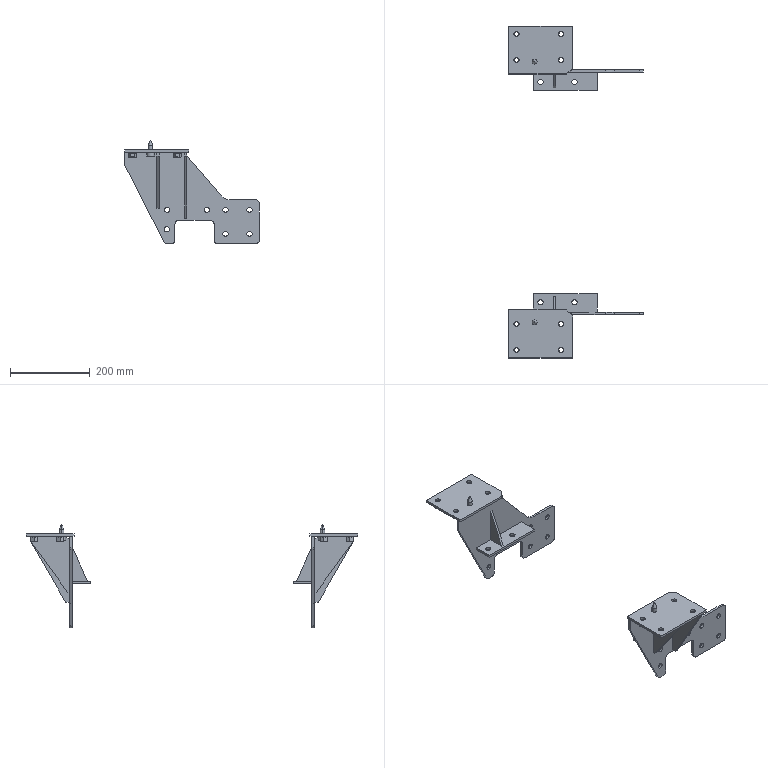Part | NX | features BREP 16 | 22 solids | 530 faces | box 337.5 x 830 x 259 mm | volume 1091429 mm3 | plane 160 | cylinder 132 | cone 118 | spline 64 | torus 56 | commonest cylinder face diameters 13 x52 12 x36 20 x22 26 x16 12.5 x4 60 x2